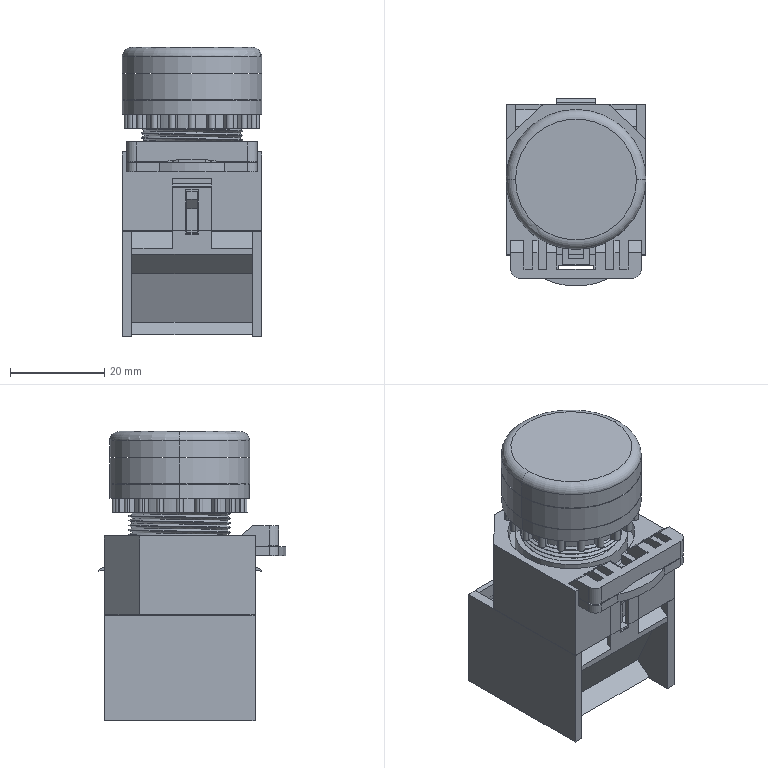Part | SolidWorks | features ICE 36, Fillet 3, MirrorPattern 3, Extrusion 1, Helix 1, Revolution 1, SweepCut 1 | 5 solids | 281 faces | box 29.7 x 39.925 x 61.4 mm | volume 43497 mm3 | plane 199 | cylinder 77 | spline 3 | torus 2 | commonest cylinder face diameters 1.5 x29 25 x20 21.6 x12 4 x4 29.7 x4 24 x2